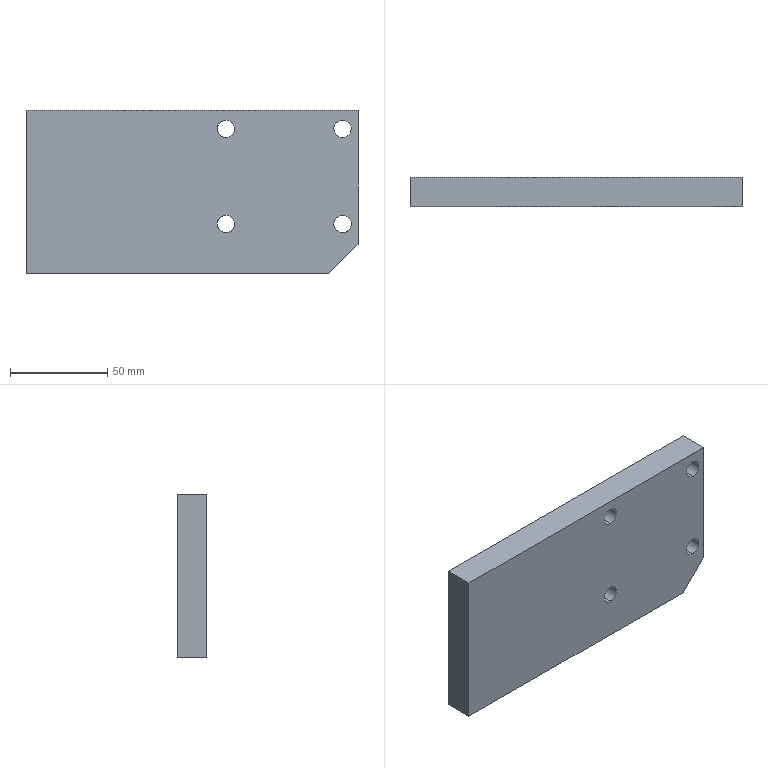Part | STEP file | Positioning_id382_x_t | 1 solid | 15 faces | box 171 x 15 x 84 mm | volume 209955 mm3 | cylinder 8 | plane 7 | commonest cylinder face diameters 9 x8